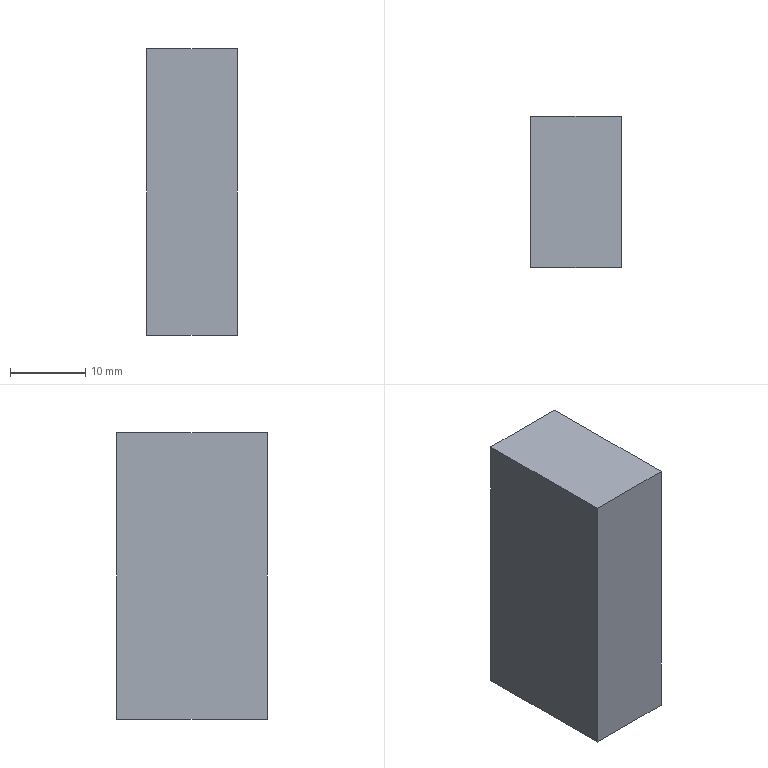Part | SolidWorks | features Extrusion 1 | 1 solid | 6 faces | box 12 x 20 x 38 mm | volume 9120 mm3 | plane 6
STEP:
#1=CARTESIAN_POINT('',(0.,20.,0.));
#2=VERTEX_POINT('',#1);
#3=CARTESIAN_POINT('',(0.,0.,0.));
#4=VERTEX_POINT('',#3);
#5=CARTESIAN_POINT('',(0.,0.,0.));
#6=DIRECTION('',(0.,-1.,0.));
#7=VECTOR('',#6,1000.);
#8=LINE('',#5,#7);
#9=EDGE_CURVE('',#2,#4,#8,.T.);
#10=ORIENTED_EDGE('',*,*,#9,.T.);
#11=CARTESIAN_POINT('',(12.,0.,0.));
#12=VERTEX_POINT('',#11);
#13=CARTESIAN_POINT('',(12.,0.,0.));
#14=DIRECTION('',(-1.,0.,0.));
#15=VECTOR('',#14,1000.);
#16=LINE('',#13,#15);
#17=EDGE_CURVE('',#12,#4,#16,.T.);
#18=ORIENTED_EDGE('',*,*,#17,.F.);
#19=CARTESIAN_POINT('',(12.,20.,0.));
#20=VERTEX_POINT('',#19);
#21=CARTESIAN_POINT('',(12.,0.,0.));
#22=DIRECTION('',(0.,-1.,0.));
#23=VECTOR('',#22,1000.);
#24=LINE('',#21,#23);
#25=EDGE_CURVE('',#20,#12,#24,.T.);
#26=ORIENTED_EDGE('',*,*,#25,.F.);
#27=CARTESIAN_POINT('',(12.,20.,0.));
#28=DIRECTION('',(-1.,0.,0.));
#29=VECTOR('',#28,1000.);
#30=LINE('',#27,#29);
#31=EDGE_CURVE('',#20,#2,#30,.T.);
#32=ORIENTED_EDGE('',*,*,#31,.T.);
#33=EDGE_LOOP('',(#10,#18,#26,#32));
#34=FACE_OUTER_BOUND('',#33,.T.);
#35=CARTESIAN_POINT('',(12.,0.,0.));
#36=DIRECTION('',(0.,0.,-1.));
#37=DIRECTION('',(-1.,0.,0.));
#38=AXIS2_PLACEMENT_3D('',#35,#36,#37);
#39=PLANE('',#38);
#40=ADVANCED_FACE('',(#34),#39,.F.);
#41=CARTESIAN_POINT('',(0.,0.,-38.));
#42=VERTEX_POINT('',#41);
#43=CARTESIAN_POINT('',(0.,0.,0.));
#44=DIRECTION('',(0.,0.,-1.));
#45=VECTOR('',#44,1000.);
#46=LINE('',#43,#45);
#47=EDGE_CURVE('',#4,#42,#46,.T.);
#48=ORIENTED_EDGE('',*,*,#47,.T.);
#49=CARTESIAN_POINT('',(12.,0.,-38.));
#50=VERTEX_POINT('',#49);
#51=CARTESIAN_POINT('',(12.,0.,-38.));
#52=DIRECTION('',(-1.,0.,0.));
#53=VECTOR('',#52,1000.);
#54=LINE('',#51,#53);
#55=EDGE_CURVE('',#50,#42,#54,.T.);
#56=ORIENTED_EDGE('',*,*,#55,.F.);
#57=CARTESIAN_POINT('',(12.,0.,0.));
#58=DIRECTION('',(0.,0.,-1.));
#59=VECTOR('',#58,1000.);
#60=LINE('',#57,#59);
#61=EDGE_CURVE('',#12,#50,#60,.T.);
#62=ORIENTED_EDGE('',*,*,#61,.F.);
#63=ORIENTED_EDGE('',*,*,#17,.T.);
#64=EDGE_LOOP('',(#48,#56,#62,#63));
#65=FACE_OUTER_BOUND('',#64,.T.);
#66=CARTESIAN_POINT('',(12.,0.,0.));
#67=DIRECTION('',(0.,1.,0.));
#68=DIRECTION('',(0.,0.,1.));
#69=AXIS2_PLACEMENT_3D('',#66,#67,#68);
#70=PLANE('',#69);
#71=ADVANCED_FACE('',(#65),#70,.F.);
#72=CARTESIAN_POINT('',(0.,20.,-38.));
#73=VERTEX_POINT('',#72);
#74=CARTESIAN_POINT('',(0.,0.,-38.));
#75=DIRECTION('',(0.,1.,0.));
#76=VECTOR('',#75,1000.);
#77=LINE('',#74,#76);
#78=EDGE_CURVE('',#42,#73,#77,.T.);
#79=ORIENTED_EDGE('',*,*,#78,.T.);
#80=CARTESIAN_POINT('',(12.,20.,-38.));
#81=VERTEX_POINT('',#80);
#82=CARTESIAN_POINT('',(12.,20.,-38.));
#83=DIRECTION('',(-1.,0.,0.));
#84=VECTOR('',#83,1000.);
#85=LINE('',#82,#84);
#86=EDGE_CURVE('',#81,#73,#85,.T.);
#87=ORIENTED_EDGE('',*,*,#86,.F.);
#88=CARTESIAN_POINT('',(12.,0.,-38.));
#89=DIRECTION('',(0.,1.,0.));
#90=VECTOR('',#89,1000.);
#91=LINE('',#88,#90);
#92=EDGE_CURVE('',#50,#81,#91,.T.);
#93=ORIENTED_EDGE('',*,*,#92,.F.);
#94=ORIENTED_EDGE('',*,*,#55,.T.);
#95=EDGE_LOOP('',(#79,#87,#93,#94));
#96=FACE_OUTER_BOUND('',#95,.T.);
#97=CARTESIAN_POINT('',(12.,0.,-38.));
#98=DIRECTION('',(0.,0.,1.));
#99=DIRECTION('',(1.,0.,0.));
#100=AXIS2_PLACEMENT_3D('',#97,#98,#99);
#101=PLANE('',#100);
#102=ADVANCED_FACE('',(#96),#101,.F.);
#103=CARTESIAN_POINT('',(0.,20.,0.));
#104=DIRECTION('',(0.,0.,1.));
#105=VECTOR('',#104,1000.);
#106=LINE('',#103,#105);
#107=EDGE_CURVE('',#73,#2,#106,.T.);
#108=ORIENTED_EDGE('',*,*,#107,.T.);
#109=ORIENTED_EDGE('',*,*,#31,.F.);
#110=CARTESIAN_POINT('',(12.,20.,0.));
#111=DIRECTION('',(0.,0.,1.));
#112=VECTOR('',#111,1000.);
#113=LINE('',#110,#112);
#114=EDGE_CURVE('',#81,#20,#113,.T.);
#115=ORIENTED_EDGE('',*,*,#114,.F.);
#116=ORIENTED_EDGE('',*,*,#86,.T.);
#117=EDGE_LOOP('',(#108,#109,#115,#116));
#118=FACE_OUTER_BOUND('',#117,.T.);
#119=CARTESIAN_POINT('',(12.,20.,0.));
#120=DIRECTION('',(0.,-1.,0.));
#121=DIRECTION('',(0.,0.,-1.));
#122=AXIS2_PLACEMENT_3D('',#119,#120,#121);
#123=PLANE('',#122);
#124=ADVANCED_FACE('',(#118),#123,.F.);
#125=ORIENTED_EDGE('',*,*,#25,.T.);
#126=ORIENTED_EDGE('',*,*,#61,.T.);
#127=ORIENTED_EDGE('',*,*,#92,.T.);
#128=ORIENTED_EDGE('',*,*,#114,.T.);
#129=EDGE_LOOP('',(#125,#126,#127,#128));
#130=FACE_OUTER_BOUND('',#129,.T.);
#131=CARTESIAN_POINT('',(12.,0.,0.));
#132=DIRECTION('',(-1.,0.,0.));
#133=DIRECTION('',(0.,0.,1.));
#134=AXIS2_PLACEMENT_3D('',#131,#132,#133);
#135=PLANE('',#134);
#136=ADVANCED_FACE('',(#130),#135,.F.);
#137=ORIENTED_EDGE('',*,*,#9,.F.);
#138=ORIENTED_EDGE('',*,*,#107,.F.);
#139=ORIENTED_EDGE('',*,*,#78,.F.);
#140=ORIENTED_EDGE('',*,*,#47,.F.);
#141=EDGE_LOOP('',(#137,#138,#139,#140));
#142=FACE_OUTER_BOUND('',#141,.T.);
#143=CARTESIAN_POINT('',(0.,0.,0.));
#144=DIRECTION('',(-1.,0.,0.));
#145=DIRECTION('',(0.,0.,1.));
#146=AXIS2_PLACEMENT_3D('',#143,#144,#145);
#147=PLANE('',#146);
#148=ADVANCED_FACE('',(#142),#147,.T.);
#149=CLOSED_SHELL('',(#40,#71,#102,#124,#136,#148));
#150=MANIFOLD_SOLID_BREP('',#149);
#151=CARTESIAN_POINT('',(0.,0.,0.));
#152=DIRECTION('',(0.,0.,1.));
#153=DIRECTION('',(1.,0.,0.));
#154=AXIS2_PLACEMENT_3D('',#151,#152,#153);
#155=(LENGTH_UNIT()NAMED_UNIT(*)SI_UNIT(.MILLI.,.METRE.));
#156=UNCERTAINTY_MEASURE_WITH_UNIT(LENGTH_MEASURE(0.00001),#155,'','');
#157=(NAMED_UNIT(*)PLANE_ANGLE_UNIT()SI_UNIT($,.RADIAN.));
#158=(NAMED_UNIT(*)SI_UNIT($,.STERADIAN.)SOLID_ANGLE_UNIT());
#159=(GEOMETRIC_REPRESENTATION_CONTEXT(3)GLOBAL_UNCERTAINTY_ASSIGNED_CONTEXT((#156))GLOBAL_UNIT_ASSIGNED_CONTEXT((#155,#157,#158))REPRESENTATION_CONTEXT('',''));
#160=ADVANCED_BREP_SHAPE_REPRESENTATION('',(#150,#154),#159);